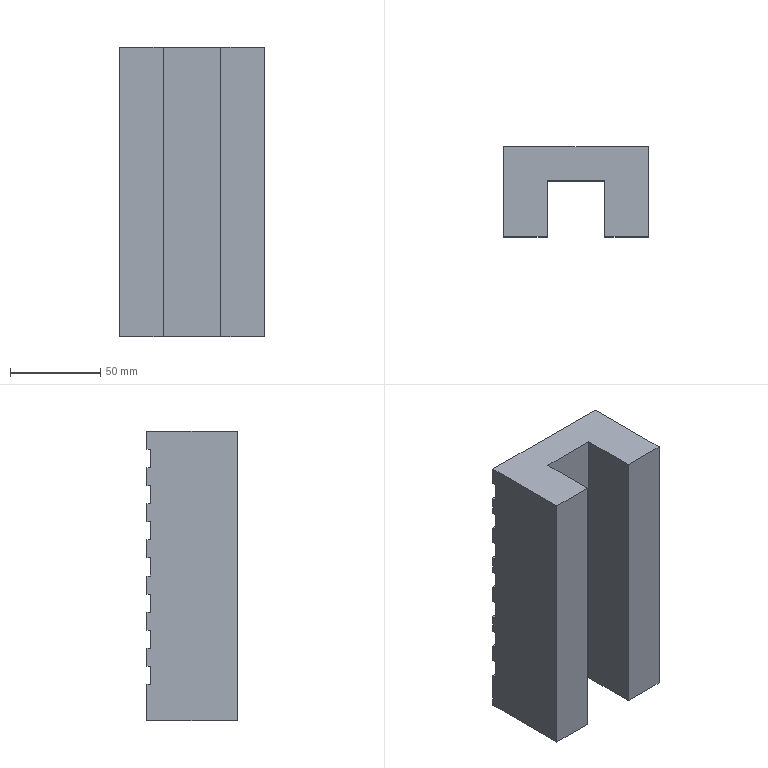Part | SolidWorks | features Extrusion 1, ICE 1, LPattern 1 | 1 solid | 38 faces | box 80 x 50 x 160 mm | volume 470080 mm3 | plane 38
STEP:
#1=CARTESIAN_POINT('',(40.,25.,40.));
#2=VERTEX_POINT('',#1);
#3=CARTESIAN_POINT('',(-40.,25.,40.));
#4=VERTEX_POINT('',#3);
#5=CARTESIAN_POINT('',(-40.,25.,40.));
#6=DIRECTION('',(-1.,0.,0.));
#7=VECTOR('',#6,1000.);
#8=LINE('',#5,#7);
#9=EDGE_CURVE('',#2,#4,#8,.T.);
#10=ORIENTED_EDGE('',*,*,#9,.F.);
#11=CARTESIAN_POINT('',(40.,25.,30.));
#12=VERTEX_POINT('',#11);
#13=CARTESIAN_POINT('',(40.,25.,160.));
#14=DIRECTION('',(0.,0.,-1.));
#15=VECTOR('',#14,1000.);
#16=LINE('',#13,#15);
#17=EDGE_CURVE('',#2,#12,#16,.T.);
#18=ORIENTED_EDGE('',*,*,#17,.T.);
#19=CARTESIAN_POINT('',(-40.,25.,30.));
#20=VERTEX_POINT('',#19);
#21=CARTESIAN_POINT('',(-40.,25.,30.));
#22=DIRECTION('',(1.,0.,0.));
#23=VECTOR('',#22,1000.);
#24=LINE('',#21,#23);
#25=EDGE_CURVE('',#20,#12,#24,.T.);
#26=ORIENTED_EDGE('',*,*,#25,.F.);
#27=CARTESIAN_POINT('',(-40.,25.,160.));
#28=DIRECTION('',(0.,0.,-1.));
#29=VECTOR('',#28,1000.);
#30=LINE('',#27,#29);
#31=EDGE_CURVE('',#4,#20,#30,.T.);
#32=ORIENTED_EDGE('',*,*,#31,.F.);
#33=EDGE_LOOP('',(#10,#18,#26,#32));
#34=FACE_OUTER_BOUND('',#33,.T.);
#35=CARTESIAN_POINT('',(0.,25.,160.));
#36=DIRECTION('',(0.,1.,0.));
#37=DIRECTION('',(-1.,0.,0.));
#38=AXIS2_PLACEMENT_3D('',#35,#36,#37);
#39=PLANE('',#38);
#40=ADVANCED_FACE('',(#34),#39,.T.);
#41=CARTESIAN_POINT('',(-40.,25.,50.));
#42=VERTEX_POINT('',#41);
#43=CARTESIAN_POINT('',(40.,25.,50.));
#44=VERTEX_POINT('',#43);
#45=CARTESIAN_POINT('',(-40.,25.,50.));
#46=DIRECTION('',(1.,0.,0.));
#47=VECTOR('',#46,1000.);
#48=LINE('',#45,#47);
#49=EDGE_CURVE('',#42,#44,#48,.T.);
#50=ORIENTED_EDGE('',*,*,#49,.F.);
#51=CARTESIAN_POINT('',(-40.,25.,60.));
#52=VERTEX_POINT('',#51);
#53=CARTESIAN_POINT('',(-40.,25.,160.));
#54=DIRECTION('',(0.,0.,-1.));
#55=VECTOR('',#54,1000.);
#56=LINE('',#53,#55);
#57=EDGE_CURVE('',#52,#42,#56,.T.);
#58=ORIENTED_EDGE('',*,*,#57,.F.);
#59=CARTESIAN_POINT('',(40.,25.,60.));
#60=VERTEX_POINT('',#59);
#61=CARTESIAN_POINT('',(-40.,25.,60.));
#62=DIRECTION('',(-1.,0.,0.));
#63=VECTOR('',#62,1000.);
#64=LINE('',#61,#63);
#65=EDGE_CURVE('',#60,#52,#64,.T.);
#66=ORIENTED_EDGE('',*,*,#65,.F.);
#67=CARTESIAN_POINT('',(40.,25.,160.));
#68=DIRECTION('',(0.,0.,-1.));
#69=VECTOR('',#68,1000.);
#70=LINE('',#67,#69);
#71=EDGE_CURVE('',#60,#44,#70,.T.);
#72=ORIENTED_EDGE('',*,*,#71,.T.);
#73=EDGE_LOOP('',(#50,#58,#66,#72));
#74=FACE_OUTER_BOUND('',#73,.T.);
#75=CARTESIAN_POINT('',(0.,25.,160.));
#76=DIRECTION('',(0.,1.,0.));
#77=DIRECTION('',(-1.,0.,0.));
#78=AXIS2_PLACEMENT_3D('',#75,#76,#77);
#79=PLANE('',#78);
#80=ADVANCED_FACE('',(#74),#79,.T.);
#81=CARTESIAN_POINT('',(-40.,25.,70.));
#82=VERTEX_POINT('',#81);
#83=CARTESIAN_POINT('',(40.,25.,70.));
#84=VERTEX_POINT('',#83);
#85=CARTESIAN_POINT('',(-40.,25.,70.));
#86=DIRECTION('',(1.,0.,0.));
#87=VECTOR('',#86,1000.);
#88=LINE('',#85,#87);
#89=EDGE_CURVE('',#82,#84,#88,.T.);
#90=ORIENTED_EDGE('',*,*,#89,.F.);
#91=CARTESIAN_POINT('',(-40.,25.,80.));
#92=VERTEX_POINT('',#91);
#93=CARTESIAN_POINT('',(-40.,25.,160.));
#94=DIRECTION('',(0.,0.,-1.));
#95=VECTOR('',#94,1000.);
#96=LINE('',#93,#95);
#97=EDGE_CURVE('',#92,#82,#96,.T.);
#98=ORIENTED_EDGE('',*,*,#97,.F.);
#99=CARTESIAN_POINT('',(40.,25.,80.));
#100=VERTEX_POINT('',#99);
#101=CARTESIAN_POINT('',(-40.,25.,80.));
#102=DIRECTION('',(-1.,0.,0.));
#103=VECTOR('',#102,1000.);
#104=LINE('',#101,#103);
#105=EDGE_CURVE('',#100,#92,#104,.T.);
#106=ORIENTED_EDGE('',*,*,#105,.F.);
#107=CARTESIAN_POINT('',(40.,25.,160.));
#108=DIRECTION('',(0.,0.,-1.));
#109=VECTOR('',#108,1000.);
#110=LINE('',#107,#109);
#111=EDGE_CURVE('',#100,#84,#110,.T.);
#112=ORIENTED_EDGE('',*,*,#111,.T.);
#113=EDGE_LOOP('',(#90,#98,#106,#112));
#114=FACE_OUTER_BOUND('',#113,.T.);
#115=CARTESIAN_POINT('',(0.,25.,160.));
#116=DIRECTION('',(0.,1.,0.));
#117=DIRECTION('',(-1.,0.,0.));
#118=AXIS2_PLACEMENT_3D('',#115,#116,#117);
#119=PLANE('',#118);
#120=ADVANCED_FACE('',(#114),#119,.T.);
#121=CARTESIAN_POINT('',(-40.,25.,90.));
#122=VERTEX_POINT('',#121);
#123=CARTESIAN_POINT('',(40.,25.,90.));
#124=VERTEX_POINT('',#123);
#125=CARTESIAN_POINT('',(-40.,25.,90.));
#126=DIRECTION('',(1.,0.,0.));
#127=VECTOR('',#126,1000.);
#128=LINE('',#125,#127);
#129=EDGE_CURVE('',#122,#124,#128,.T.);
#130=ORIENTED_EDGE('',*,*,#129,.F.);
#131=CARTESIAN_POINT('',(-40.,25.,100.));
#132=VERTEX_POINT('',#131);
#133=CARTESIAN_POINT('',(-40.,25.,160.));
#134=DIRECTION('',(0.,0.,-1.));
#135=VECTOR('',#134,1000.);
#136=LINE('',#133,#135);
#137=EDGE_CURVE('',#132,#122,#136,.T.);
#138=ORIENTED_EDGE('',*,*,#137,.F.);
#139=CARTESIAN_POINT('',(40.,25.,100.));
#140=VERTEX_POINT('',#139);
#141=CARTESIAN_POINT('',(-40.,25.,100.));
#142=DIRECTION('',(-1.,0.,0.));
#143=VECTOR('',#142,1000.);
#144=LINE('',#141,#143);
#145=EDGE_CURVE('',#140,#132,#144,.T.);
#146=ORIENTED_EDGE('',*,*,#145,.F.);
#147=CARTESIAN_POINT('',(40.,25.,160.));
#148=DIRECTION('',(0.,0.,-1.));
#149=VECTOR('',#148,1000.);
#150=LINE('',#147,#149);
#151=EDGE_CURVE('',#140,#124,#150,.T.);
#152=ORIENTED_EDGE('',*,*,#151,.T.);
#153=EDGE_LOOP('',(#130,#138,#146,#152));
#154=FACE_OUTER_BOUND('',#153,.T.);
#155=CARTESIAN_POINT('',(0.,25.,160.));
#156=DIRECTION('',(0.,1.,0.));
#157=DIRECTION('',(-1.,0.,0.));
#158=AXIS2_PLACEMENT_3D('',#155,#156,#157);
#159=PLANE('',#158);
#160=ADVANCED_FACE('',(#154),#159,.T.);
#161=CARTESIAN_POINT('',(-40.,25.,110.));
#162=VERTEX_POINT('',#161);
#163=CARTESIAN_POINT('',(40.,25.,110.));
#164=VERTEX_POINT('',#163);
#165=CARTESIAN_POINT('',(-40.,25.,110.));
#166=DIRECTION('',(1.,0.,0.));
#167=VECTOR('',#166,1000.);
#168=LINE('',#165,#167);
#169=EDGE_CURVE('',#162,#164,#168,.T.);
#170=ORIENTED_EDGE('',*,*,#169,.F.);
#171=CARTESIAN_POINT('',(-40.,25.,120.));
#172=VERTEX_POINT('',#171);
#173=CARTESIAN_POINT('',(-40.,25.,160.));
#174=DIRECTION('',(0.,0.,-1.));
#175=VECTOR('',#174,1000.);
#176=LINE('',#173,#175);
#177=EDGE_CURVE('',#172,#162,#176,.T.);
#178=ORIENTED_EDGE('',*,*,#177,.F.);
#179=CARTESIAN_POINT('',(40.,25.,120.));
#180=VERTEX_POINT('',#179);
#181=CARTESIAN_POINT('',(-40.,25.,120.));
#182=DIRECTION('',(-1.,0.,0.));
#183=VECTOR('',#182,1000.);
#184=LINE('',#181,#183);
#185=EDGE_CURVE('',#180,#172,#184,.T.);
#186=ORIENTED_EDGE('',*,*,#185,.F.);
#187=CARTESIAN_POINT('',(40.,25.,160.));
#188=DIRECTION('',(0.,0.,-1.));
#189=VECTOR('',#188,1000.);
#190=LINE('',#187,#189);
#191=EDGE_CURVE('',#180,#164,#190,.T.);
#192=ORIENTED_EDGE('',*,*,#191,.T.);
#193=EDGE_LOOP('',(#170,#178,#186,#192));
#194=FACE_OUTER_BOUND('',#193,.T.);
#195=CARTESIAN_POINT('',(0.,25.,160.));
#196=DIRECTION('',(0.,1.,0.));
#197=DIRECTION('',(-1.,0.,0.));
#198=AXIS2_PLACEMENT_3D('',#195,#196,#197);
#199=PLANE('',#198);
#200=ADVANCED_FACE('',(#194),#199,.T.);
#201=CARTESIAN_POINT('',(-40.,25.,130.));
#202=VERTEX_POINT('',#201);
#203=CARTESIAN_POINT('',(40.,25.,130.));
#204=VERTEX_POINT('',#203);
#205=CARTESIAN_POINT('',(-40.,25.,130.));
#206=DIRECTION('',(1.,0.,0.));
#207=VECTOR('',#206,1000.);
#208=LINE('',#205,#207);
#209=EDGE_CURVE('',#202,#204,#208,.T.);
#210=ORIENTED_EDGE('',*,*,#209,.F.);
#211=CARTESIAN_POINT('',(-40.,25.,140.));
#212=VERTEX_POINT('',#211);
#213=CARTESIAN_POINT('',(-40.,25.,160.));
#214=DIRECTION('',(0.,0.,-1.));
#215=VECTOR('',#214,1000.);
#216=LINE('',#213,#215);
#217=EDGE_CURVE('',#212,#202,#216,.T.);
#218=ORIENTED_EDGE('',*,*,#217,.F.);
#219=CARTESIAN_POINT('',(40.,25.,140.));
#220=VERTEX_POINT('',#219);
#221=CARTESIAN_POINT('',(-40.,25.,140.));
#222=DIRECTION('',(-1.,0.,0.));
#223=VECTOR('',#222,1000.);
#224=LINE('',#221,#223);
#225=EDGE_CURVE('',#220,#212,#224,.T.);
#226=ORIENTED_EDGE('',*,*,#225,.F.);
#227=CARTESIAN_POINT('',(40.,25.,160.));
#228=DIRECTION('',(0.,0.,-1.));
#229=VECTOR('',#228,1000.);
#230=LINE('',#227,#229);
#231=EDGE_CURVE('',#220,#204,#230,.T.);
#232=ORIENTED_EDGE('',*,*,#231,.T.);
#233=EDGE_LOOP('',(#210,#218,#226,#232));
#234=FACE_OUTER_BOUND('',#233,.T.);
#235=CARTESIAN_POINT('',(0.,25.,160.));
#236=DIRECTION('',(0.,1.,0.));
#237=DIRECTION('',(-1.,0.,0.));
#238=AXIS2_PLACEMENT_3D('',#235,#236,#237);
#239=PLANE('',#238);
#240=ADVANCED_FACE('',(#234),#239,.T.);
#241=CARTESIAN_POINT('',(40.,25.,20.));
#242=VERTEX_POINT('',#241);
#243=CARTESIAN_POINT('',(-40.,25.,20.));
#244=VERTEX_POINT('',#243);
#245=CARTESIAN_POINT('',(-40.,25.,20.));
#246=DIRECTION('',(-1.,0.,0.));
#247=VECTOR('',#246,1000.);
#248=LINE('',#245,#247);
#249=EDGE_CURVE('',#242,#244,#248,.T.);
#250=ORIENTED_EDGE('',*,*,#249,.F.);
#251=CARTESIAN_POINT('',(40.,25.,0.));
#252=VERTEX_POINT('',#251);
#253=CARTESIAN_POINT('',(40.,25.,160.));
#254=DIRECTION('',(0.,0.,-1.));
#255=VECTOR('',#254,1000.);
#256=LINE('',#253,#255);
#257=EDGE_CURVE('',#242,#252,#256,.T.);
#258=ORIENTED_EDGE('',*,*,#257,.T.);
#259=CARTESIAN_POINT('',(-40.,25.,0.));
#260=VERTEX_POINT('',#259);
#261=CARTESIAN_POINT('',(0.,25.,0.));
#262=DIRECTION('',(1.,0.,0.));
#263=VECTOR('',#262,1000.);
#264=LINE('',#261,#263);
#265=EDGE_CURVE('',#260,#252,#264,.T.);
#266=ORIENTED_EDGE('',*,*,#265,.F.);
#267=CARTESIAN_POINT('',(-40.,25.,160.));
#268=DIRECTION('',(0.,0.,-1.));
#269=VECTOR('',#268,1000.);
#270=LINE('',#267,#269);
#271=EDGE_CURVE('',#244,#260,#270,.T.);
#272=ORIENTED_EDGE('',*,*,#271,.F.);
#273=EDGE_LOOP('',(#250,#258,#266,#272));
#274=FACE_OUTER_BOUND('',#273,.T.);
#275=CARTESIAN_POINT('',(0.,25.,160.));
#276=DIRECTION('',(0.,1.,0.));
#277=DIRECTION('',(-1.,0.,0.));
#278=AXIS2_PLACEMENT_3D('',#275,#276,#277);
#279=PLANE('',#278);
#280=ADVANCED_FACE('',(#274),#279,.T.);
#281=CARTESIAN_POINT('',(-16.,-25.,0.));
#282=VERTEX_POINT('',#281);
#283=CARTESIAN_POINT('',(-16.,6.,0.));
#284=VERTEX_POINT('',#283);
#285=CARTESIAN_POINT('',(-16.,0.,0.));
#286=DIRECTION('',(0.,1.,0.));
#287=VECTOR('',#286,1000.);
#288=LINE('',#285,#287);
#289=EDGE_CURVE('',#282,#284,#288,.T.);
#290=ORIENTED_EDGE('',*,*,#289,.T.);
#291=CARTESIAN_POINT('',(-16.,6.,160.));
#292=VERTEX_POINT('',#291);
#293=CARTESIAN_POINT('',(-16.,6.,160.));
#294=DIRECTION('',(0.,0.,-1.));
#295=VECTOR('',#294,1000.);
#296=LINE('',#293,#295);
#297=EDGE_CURVE('',#292,#284,#296,.T.);
#298=ORIENTED_EDGE('',*,*,#297,.F.);
#299=CARTESIAN_POINT('',(-16.,-25.,160.));
#300=VERTEX_POINT('',#299);
#301=CARTESIAN_POINT('',(-16.,0.,160.));
#302=DIRECTION('',(0.,1.,0.));
#303=VECTOR('',#302,1000.);
#304=LINE('',#301,#303);
#305=EDGE_CURVE('',#300,#292,#304,.T.);
#306=ORIENTED_EDGE('',*,*,#305,.F.);
#307=CARTESIAN_POINT('',(-16.,-25.,160.));
#308=DIRECTION('',(0.,0.,-1.));
#309=VECTOR('',#308,1000.);
#310=LINE('',#307,#309);
#311=EDGE_CURVE('',#300,#282,#310,.T.);
#312=ORIENTED_EDGE('',*,*,#311,.T.);
#313=EDGE_LOOP('',(#290,#298,#306,#312));
#314=FACE_OUTER_BOUND('',#313,.T.);
#315=CARTESIAN_POINT('',(-16.,0.,160.));
#316=DIRECTION('',(-1.,0.,0.));
#317=DIRECTION('',(0.,0.,1.));
#318=AXIS2_PLACEMENT_3D('',#315,#316,#317);
#319=PLANE('',#318);
#320=ADVANCED_FACE('',(#314),#319,.F.);
#321=CARTESIAN_POINT('',(16.,6.,0.));
#322=VERTEX_POINT('',#321);
#323=CARTESIAN_POINT('',(0.,6.,0.));
#324=DIRECTION('',(1.,0.,0.));
#325=VECTOR('',#324,1000.);
#326=LINE('',#323,#325);
#327=EDGE_CURVE('',#284,#322,#326,.T.);
#328=ORIENTED_EDGE('',*,*,#327,.T.);
#329=CARTESIAN_POINT('',(16.,6.,160.));
#330=VERTEX_POINT('',#329);
#331=CARTESIAN_POINT('',(16.,6.,160.));
#332=DIRECTION('',(0.,0.,-1.));
#333=VECTOR('',#332,1000.);
#334=LINE('',#331,#333);
#335=EDGE_CURVE('',#330,#322,#334,.T.);
#336=ORIENTED_EDGE('',*,*,#335,.F.);
#337=CARTESIAN_POINT('',(0.,6.,160.));
#338=DIRECTION('',(1.,0.,0.));
#339=VECTOR('',#338,1000.);
#340=LINE('',#337,#339);
#341=EDGE_CURVE('',#292,#330,#340,.T.);
#342=ORIENTED_EDGE('',*,*,#341,.F.);
#343=ORIENTED_EDGE('',*,*,#297,.T.);
#344=EDGE_LOOP('',(#328,#336,#342,#343));
#345=FACE_OUTER_BOUND('',#344,.T.);
#346=CARTESIAN_POINT('',(0.,6.,160.));
#347=DIRECTION('',(0.,1.,0.));
#348=DIRECTION('',(-1.,0.,0.));
#349=AXIS2_PLACEMENT_3D('',#346,#347,#348);
#350=PLANE('',#349);
#351=ADVANCED_FACE('',(#345),#350,.F.);
#352=CARTESIAN_POINT('',(16.,-25.,0.));
#353=VERTEX_POINT('',#352);
#354=CARTESIAN_POINT('',(16.,0.,0.));
#355=DIRECTION('',(0.,1.,0.));
#356=VECTOR('',#355,1000.);
#357=LINE('',#354,#356);
#358=EDGE_CURVE('',#353,#322,#357,.T.);
#359=ORIENTED_EDGE('',*,*,#358,.F.);
#360=CARTESIAN_POINT('',(16.,-25.,160.));
#361=VERTEX_POINT('',#360);
#362=CARTESIAN_POINT('',(16.,-25.,160.));
#363=DIRECTION('',(0.,0.,-1.));
#364=VECTOR('',#363,1000.);
#365=LINE('',#362,#364);
#366=EDGE_CURVE('',#361,#353,#365,.T.);
#367=ORIENTED_EDGE('',*,*,#366,.F.);
#368=CARTESIAN_POINT('',(16.,0.,160.));
#369=DIRECTION('',(0.,1.,0.));
#370=VECTOR('',#369,1000.);
#371=LINE('',#368,#370);
#372=EDGE_CURVE('',#361,#330,#371,.T.);
#373=ORIENTED_EDGE('',*,*,#372,.T.);
#374=ORIENTED_EDGE('',*,*,#335,.T.);
#375=EDGE_LOOP('',(#359,#367,#373,#374));
#376=FACE_OUTER_BOUND('',#375,.T.);
#377=CARTESIAN_POINT('',(16.,0.,160.));
#378=DIRECTION('',(-1.,0.,0.));
#379=DIRECTION('',(0.,-1.,0.));
#380=AXIS2_PLACEMENT_3D('',#377,#378,#379);
#381=PLANE('',#380);
#382=ADVANCED_FACE('',(#376),#381,.T.);
#383=CARTESIAN_POINT('',(40.,-25.,0.));
#384=VERTEX_POINT('',#383);
#385=CARTESIAN_POINT('',(0.,-25.,0.));
#386=DIRECTION('',(1.,0.,0.));
#387=VECTOR('',#386,1000.);
#388=LINE('',#385,#387);
#389=EDGE_CURVE('',#353,#384,#388,.T.);
#390=ORIENTED_EDGE('',*,*,#389,.T.);
#391=CARTESIAN_POINT('',(40.,-25.,160.));
#392=VERTEX_POINT('',#391);
#393=CARTESIAN_POINT('',(40.,-25.,160.));
#394=DIRECTION('',(0.,0.,-1.));
#395=VECTOR('',#394,1000.);
#396=LINE('',#393,#395);
#397=EDGE_CURVE('',#392,#384,#396,.T.);
#398=ORIENTED_EDGE('',*,*,#397,.F.);
#399=CARTESIAN_POINT('',(0.,-25.,160.));
#400=DIRECTION('',(1.,0.,0.));
#401=VECTOR('',#400,1000.);
#402=LINE('',#399,#401);
#403=EDGE_CURVE('',#361,#392,#402,.T.);
#404=ORIENTED_EDGE('',*,*,#403,.F.);
#405=ORIENTED_EDGE('',*,*,#366,.T.);
#406=EDGE_LOOP('',(#390,#398,#404,#405));
#407=FACE_OUTER_BOUND('',#406,.T.);
#408=CARTESIAN_POINT('',(0.,-25.,160.));
#409=DIRECTION('',(0.,1.,0.));
#410=DIRECTION('',(-1.,0.,0.));
#411=AXIS2_PLACEMENT_3D('',#408,#409,#410);
#412=PLANE('',#411);
#413=ADVANCED_FACE('',(#407),#412,.F.);
#414=CARTESIAN_POINT('',(40.,23.,40.));
#415=VERTEX_POINT('',#414);
#416=CARTESIAN_POINT('',(40.,23.,40.));
#417=DIRECTION('',(0.,1.,0.));
#418=VECTOR('',#417,1000.);
#419=LINE('',#416,#418);
#420=EDGE_CURVE('',#415,#2,#419,.T.);
#421=ORIENTED_EDGE('',*,*,#420,.F.);
#422=CARTESIAN_POINT('',(40.,23.,50.));
#423=VERTEX_POINT('',#422);
#424=CARTESIAN_POINT('',(40.,23.,40.));
#425=DIRECTION('',(0.,0.,-1.));
#426=VECTOR('',#425,1000.);
#427=LINE('',#424,#426);
#428=EDGE_CURVE('',#423,#415,#427,.T.);
#429=ORIENTED_EDGE('',*,*,#428,.F.);
#430=CARTESIAN_POINT('',(40.,23.,50.));
#431=DIRECTION('',(0.,1.,0.));
#432=VECTOR('',#431,1000.);
#433=LINE('',#430,#432);
#434=EDGE_CURVE('',#423,#44,#433,.T.);
#435=ORIENTED_EDGE('',*,*,#434,.T.);
#436=ORIENTED_EDGE('',*,*,#71,.F.);
#437=CARTESIAN_POINT('',(40.,23.,60.));
#438=VERTEX_POINT('',#437);
#439=CARTESIAN_POINT('',(40.,23.,60.));
#440=DIRECTION('',(0.,1.,0.));
#441=VECTOR('',#440,1000.);
#442=LINE('',#439,#441);
#443=EDGE_CURVE('',#438,#60,#442,.T.);
#444=ORIENTED_EDGE('',*,*,#443,.F.);
#445=CARTESIAN_POINT('',(40.,23.,70.));
#446=VERTEX_POINT('',#445);
#447=CARTESIAN_POINT('',(40.,23.,60.));
#448=DIRECTION('',(0.,0.,-1.));
#449=VECTOR('',#448,1000.);
#450=LINE('',#447,#449);
#451=EDGE_CURVE('',#446,#438,#450,.T.);
#452=ORIENTED_EDGE('',*,*,#451,.F.);
#453=CARTESIAN_POINT('',(40.,23.,70.));
#454=DIRECTION('',(0.,1.,0.));
#455=VECTOR('',#454,1000.);
#456=LINE('',#453,#455);
#457=EDGE_CURVE('',#446,#84,#456,.T.);
#458=ORIENTED_EDGE('',*,*,#457,.T.);
#459=ORIENTED_EDGE('',*,*,#111,.F.);
#460=CARTESIAN_POINT('',(40.,23.,80.));
#461=VERTEX_POINT('',#460);
#462=CARTESIAN_POINT('',(40.,23.,80.));
#463=DIRECTION('',(0.,1.,0.));
#464=VECTOR('',#463,1000.);
#465=LINE('',#462,#464);
#466=EDGE_CURVE('',#461,#100,#465,.T.);
#467=ORIENTED_EDGE('',*,*,#466,.F.);
#468=CARTESIAN_POINT('',(40.,23.,90.));
#469=VERTEX_POINT('',#468);
#470=CARTESIAN_POINT('',(40.,23.,80.));
#471=DIRECTION('',(0.,0.,-1.));
#472=VECTOR('',#471,1000.);
#473=LINE('',#470,#472);
#474=EDGE_CURVE('',#469,#461,#473,.T.);
#475=ORIENTED_EDGE('',*,*,#474,.F.);
#476=CARTESIAN_POINT('',(40.,23.,90.));
#477=DIRECTION('',(0.,1.,0.));
#478=VECTOR('',#477,1000.);
#479=LINE('',#476,#478);
#480=EDGE_CURVE('',#469,#124,#479,.T.);
#481=ORIENTED_EDGE('',*,*,#480,.T.);
#482=ORIENTED_EDGE('',*,*,#151,.F.);
#483=CARTESIAN_POINT('',(40.,23.,100.));
#484=VERTEX_POINT('',#483);
#485=CARTESIAN_POINT('',(40.,23.,100.));
#486=DIRECTION('',(0.,1.,0.));
#487=VECTOR('',#486,1000.);
#488=LINE('',#485,#487);
#489=EDGE_CURVE('',#484,#140,#488,.T.);
#490=ORIENTED_EDGE('',*,*,#489,.F.);
#491=CARTESIAN_POINT('',(40.,23.,110.));
#492=VERTEX_POINT('',#491);
#493=CARTESIAN_POINT('',(40.,23.,100.));
#494=DIRECTION('',(0.,0.,-1.));
#495=VECTOR('',#494,1000.);
#496=LINE('',#493,#495);
#497=EDGE_CURVE('',#492,#484,#496,.T.);
#498=ORIENTED_EDGE('',*,*,#497,.F.);
#499=CARTESIAN_POINT('',(40.,23.,110.));
#500=DIRECTION('',(0.,1.,0.));
#501=VECTOR('',#500,1000.);
#502=LINE('',#499,#501);
#503=EDGE_CURVE('',#492,#164,#502,.T.);
#504=ORIENTED_EDGE('',*,*,#503,.T.);
#505=ORIENTED_EDGE('',*,*,#191,.F.);
#506=CARTESIAN_POINT('',(40.,23.,120.));
#507=VERTEX_POINT('',#506);
#508=CARTESIAN_POINT('',(40.,23.,120.));
#509=DIRECTION('',(0.,1.,0.));
#510=VECTOR('',#509,1000.);
#511=LINE('',#508,#510);
#512=EDGE_CURVE('',#507,#180,#511,.T.);
#513=ORIENTED_EDGE('',*,*,#512,.F.);
#514=CARTESIAN_POINT('',(40.,23.,130.));
#515=VERTEX_POINT('',#514);
#516=CARTESIAN_POINT('',(40.,23.,120.));
#517=DIRECTION('',(0.,0.,-1.));
#518=VECTOR('',#517,1000.);
#519=LINE('',#516,#518);
#520=EDGE_CURVE('',#515,#507,#519,.T.);
#521=ORIENTED_EDGE('',*,*,#520,.F.);
#522=CARTESIAN_POINT('',(40.,23.,130.));
#523=DIRECTION('',(0.,1.,0.));
#524=VECTOR('',#523,1000.);
#525=LINE('',#522,#524);
#526=EDGE_CURVE('',#515,#204,#525,.T.);
#527=ORIENTED_EDGE('',*,*,#526,.T.);
#528=ORIENTED_EDGE('',*,*,#231,.F.);
#529=CARTESIAN_POINT('',(40.,23.,140.));
#530=VERTEX_POINT('',#529);
#531=CARTESIAN_POINT('',(40.,23.,140.));
#532=DIRECTION('',(0.,1.,0.));
#533=VECTOR('',#532,1000.);
#534=LINE('',#531,#533);
#535=EDGE_CURVE('',#530,#220,#534,.T.);
#536=ORIENTED_EDGE('',*,*,#535,.F.);
#537=CARTESIAN_POINT('',(40.,23.,150.));
#538=VERTEX_POINT('',#537);
#539=CARTESIAN_POINT('',(40.,23.,140.));
#540=DIRECTION('',(0.,0.,-1.));
#541=VECTOR('',#540,1000.);
#542=LINE('',#539,#541);
#543=EDGE_CURVE('',#538,#530,#542,.T.);
#544=ORIENTED_EDGE('',*,*,#543,.F.);
#545=CARTESIAN_POINT('',(40.,25.,150.));
#546=VERTEX_POINT('',#545);
#547=CARTESIAN_POINT('',(40.,23.,150.));
#548=DIRECTION('',(0.,1.,0.));
#549=VECTOR('',#548,1000.);
#550=LINE('',#547,#549);
#551=EDGE_CURVE('',#538,#546,#550,.T.);
#552=ORIENTED_EDGE('',*,*,#551,.T.);
#553=CARTESIAN_POINT('',(40.,25.,160.));
#554=VERTEX_POINT('',#553);
#555=CARTESIAN_POINT('',(40.,25.,160.));
#556=DIRECTION('',(0.,0.,-1.));
#557=VECTOR('',#556,1000.);
#558=LINE('',#555,#557);
#559=EDGE_CURVE('',#554,#546,#558,.T.);
#560=ORIENTED_EDGE('',*,*,#559,.F.);
#561=CARTESIAN_POINT('',(40.,0.,160.));
#562=DIRECTION('',(0.,-1.,0.));
#563=VECTOR('',#562,1000.);
#564=LINE('',#561,#563);
#565=EDGE_CURVE('',#554,#392,#564,.T.);
#566=ORIENTED_EDGE('',*,*,#565,.T.);
#567=ORIENTED_EDGE('',*,*,#397,.T.);
#568=CARTESIAN_POINT('',(40.,0.,0.));
#569=DIRECTION('',(0.,-1.,0.));
#570=VECTOR('',#569,1000.);
#571=LINE('',#568,#570);
#572=EDGE_CURVE('',#252,#384,#571,.T.);
#573=ORIENTED_EDGE('',*,*,#572,.F.);
#574=ORIENTED_EDGE('',*,*,#257,.F.);
#575=CARTESIAN_POINT('',(40.,23.,20.));
#576=VERTEX_POINT('',#575);
#577=CARTESIAN_POINT('',(40.,23.,20.));
#578=DIRECTION('',(0.,1.,0.));
#579=VECTOR('',#578,1000.);
#580=LINE('',#577,#579);
#581=EDGE_CURVE('',#576,#242,#580,.T.);
#582=ORIENTED_EDGE('',*,*,#581,.F.);
#583=CARTESIAN_POINT('',(40.,23.,30.));
#584=VERTEX_POINT('',#583);
#585=CARTESIAN_POINT('',(40.,23.,20.));
#586=DIRECTION('',(0.,0.,-1.));
#587=VECTOR('',#586,1000.);
#588=LINE('',#585,#587);
#589=EDGE_CURVE('',#584,#576,#588,.T.);
#590=ORIENTED_EDGE('',*,*,#589,.F.);
#591=CARTESIAN_POINT('',(40.,23.,30.));
#592=DIRECTION('',(0.,1.,0.));
#593=VECTOR('',#592,1000.);
#594=LINE('',#591,#593);
#595=EDGE_CURVE('',#584,#12,#594,.T.);
#596=ORIENTED_EDGE('',*,*,#595,.T.);
#597=ORIENTED_EDGE('',*,*,#17,.F.);
#598=EDGE_LOOP('',(#421,#429,#435,#436,#444,#452,#458,#459,#467,#475,#481,#482,#490,#498,#504,#505,#513,#521,#527,#528,#536,#544,#552,#560,#566,#567,#573,#574,#582,#590,#596,#597));
#599=FACE_OUTER_BOUND('',#598,.T.);
#600=CARTESIAN_POINT('',(40.,0.,160.));
#601=DIRECTION('',(1.,0.,0.));
#602=DIRECTION('',(0.,1.,0.));
#603=AXIS2_PLACEMENT_3D('',#600,#601,#602);
#604=PLANE('',#603);
#605=ADVANCED_FACE('',(#599),#604,.T.);
#606=CARTESIAN_POINT('',(-40.,25.,150.));
#607=VERTEX_POINT('',#606);
#608=CARTESIAN_POINT('',(-40.,25.,150.));
#609=DIRECTION('',(1.,0.,0.));
#610=VECTOR('',#609,1000.);
#611=LINE('',#608,#610);
#612=EDGE_CURVE('',#607,#546,#611,.T.);
#613=ORIENTED_EDGE('',*,*,#612,.F.);
#614=CARTESIAN_POINT('',(-40.,25.,160.));
#615=VERTEX_POINT('',#614);
#616=CARTESIAN_POINT('',(-40.,25.,160.));
#617=DIRECTION('',(0.,0.,-1.));
#618=VECTOR('',#617,1000.);
#619=LINE('',#616,#618);
#620=EDGE_CURVE('',#615,#607,#619,.T.);
#621=ORIENTED_EDGE('',*,*,#620,.F.);
#622=CARTESIAN_POINT('',(0.,25.,160.));
#623=DIRECTION('',(1.,0.,0.));
#624=VECTOR('',#623,1000.);
#625=LINE('',#622,#624);
#626=EDGE_CURVE('',#615,#554,#625,.T.);
#627=ORIENTED_EDGE('',*,*,#626,.T.);
#628=ORIENTED_EDGE('',*,*,#559,.T.);
#629=EDGE_LOOP('',(#613,#621,#627,#628));
#630=FACE_OUTER_BOUND('',#629,.T.);
#631=CARTESIAN_POINT('',(0.,25.,160.));
#632=DIRECTION('',(0.,1.,0.));
#633=DIRECTION('',(-1.,0.,0.));
#634=AXIS2_PLACEMENT_3D('',#631,#632,#633);
#635=PLANE('',#634);
#636=ADVANCED_FACE('',(#630),#635,.T.);
#637=CARTESIAN_POINT('',(-40.,23.,40.));
#638=VERTEX_POINT('',#637);
#639=CARTESIAN_POINT('',(-40.,23.,50.));
#640=VERTEX_POINT('',#639);
#641=CARTESIAN_POINT('',(-40.,23.,40.));
#642=DIRECTION('',(0.,0.,1.));
#643=VECTOR('',#642,1000.);
#644=LINE('',#641,#643);
#645=EDGE_CURVE('',#638,#640,#644,.T.);
#646=ORIENTED_EDGE('',*,*,#645,.F.);
#647=CARTESIAN_POINT('',(-40.,23.,40.));
#648=DIRECTION('',(0.,1.,0.));
#649=VECTOR('',#648,1000.);
#650=LINE('',#647,#649);
#651=EDGE_CURVE('',#638,#4,#650,.T.);
#652=ORIENTED_EDGE('',*,*,#651,.T.);
#653=ORIENTED_EDGE('',*,*,#31,.T.);
#654=CARTESIAN_POINT('',(-40.,23.,30.));
#655=VERTEX_POINT('',#654);
#656=CARTESIAN_POINT('',(-40.,23.,30.));
#657=DIRECTION('',(0.,1.,0.));
#658=VECTOR('',#657,1000.);
#659=LINE('',#656,#658);
#660=EDGE_CURVE('',#655,#20,#659,.T.);
#661=ORIENTED_EDGE('',*,*,#660,.F.);
#662=CARTESIAN_POINT('',(-40.,23.,20.));
#663=VERTEX_POINT('',#662);
#664=CARTESIAN_POINT('',(-40.,23.,20.));
#665=DIRECTION('',(0.,0.,1.));
#666=VECTOR('',#665,1000.);
#667=LINE('',#664,#666);
#668=EDGE_CURVE('',#663,#655,#667,.T.);
#669=ORIENTED_EDGE('',*,*,#668,.F.);
#670=CARTESIAN_POINT('',(-40.,23.,20.));
#671=DIRECTION('',(0.,1.,0.));
#672=VECTOR('',#671,1000.);
#673=LINE('',#670,#672);
#674=EDGE_CURVE('',#663,#244,#673,.T.);
#675=ORIENTED_EDGE('',*,*,#674,.T.);
#676=ORIENTED_EDGE('',*,*,#271,.T.);
#677=CARTESIAN_POINT('',(-40.,-25.,0.));
#678=VERTEX_POINT('',#677);
#679=CARTESIAN_POINT('',(-40.,0.,0.));
#680=DIRECTION('',(0.,-1.,0.));
#681=VECTOR('',#680,1000.);
#682=LINE('',#679,#681);
#683=EDGE_CURVE('',#260,#678,#682,.T.);
#684=ORIENTED_EDGE('',*,*,#683,.T.);
#685=CARTESIAN_POINT('',(-40.,-25.,160.));
#686=VERTEX_POINT('',#685);
#687=CARTESIAN_POINT('',(-40.,-25.,160.));
#688=DIRECTION('',(0.,0.,-1.));
#689=VECTOR('',#688,1000.);
#690=LINE('',#687,#689);
#691=EDGE_CURVE('',#686,#678,#690,.T.);
#692=ORIENTED_EDGE('',*,*,#691,.F.);
#693=CARTESIAN_POINT('',(-40.,0.,160.));
#694=DIRECTION('',(0.,-1.,0.));
#695=VECTOR('',#694,1000.);
#696=LINE('',#693,#695);
#697=EDGE_CURVE('',#615,#686,#696,.T.);
#698=ORIENTED_EDGE('',*,*,#697,.F.);
#699=ORIENTED_EDGE('',*,*,#620,.T.);
#700=CARTESIAN_POINT('',(-40.,23.,150.));
#701=VERTEX_POINT('',#700);
#702=CARTESIAN_POINT('',(-40.,23.,150.));
#703=DIRECTION('',(0.,1.,0.));
#704=VECTOR('',#703,1000.);
#705=LINE('',#702,#704);
#706=EDGE_CURVE('',#701,#607,#705,.T.);
#707=ORIENTED_EDGE('',*,*,#706,.F.);
#708=CARTESIAN_POINT('',(-40.,23.,140.));
#709=VERTEX_POINT('',#708);
#710=CARTESIAN_POINT('',(-40.,23.,140.));
#711=DIRECTION('',(0.,0.,1.));
#712=VECTOR('',#711,1000.);
#713=LINE('',#710,#712);
#714=EDGE_CURVE('',#709,#701,#713,.T.);
#715=ORIENTED_EDGE('',*,*,#714,.F.);
#716=CARTESIAN_POINT('',(-40.,23.,140.));
#717=DIRECTION('',(0.,1.,0.));
#718=VECTOR('',#717,1000.);
#719=LINE('',#716,#718);
#720=EDGE_CURVE('',#709,#212,#719,.T.);
#721=ORIENTED_EDGE('',*,*,#720,.T.);
#722=ORIENTED_EDGE('',*,*,#217,.T.);
#723=CARTESIAN_POINT('',(-40.,23.,130.));
#724=VERTEX_POINT('',#723);
#725=CARTESIAN_POINT('',(-40.,23.,130.));
#726=DIRECTION('',(0.,1.,0.));
#727=VECTOR('',#726,1000.);
#728=LINE('',#725,#727);
#729=EDGE_CURVE('',#724,#202,#728,.T.);
#730=ORIENTED_EDGE('',*,*,#729,.F.);
#731=CARTESIAN_POINT('',(-40.,23.,120.));
#732=VERTEX_POINT('',#731);
#733=CARTESIAN_POINT('',(-40.,23.,120.));
#734=DIRECTION('',(0.,0.,1.));
#735=VECTOR('',#734,1000.);
#736=LINE('',#733,#735);
#737=EDGE_CURVE('',#732,#724,#736,.T.);
#738=ORIENTED_EDGE('',*,*,#737,.F.);
#739=CARTESIAN_POINT('',(-40.,23.,120.));
#740=DIRECTION('',(0.,1.,0.));
#741=VECTOR('',#740,1000.);
#742=LINE('',#739,#741);
#743=EDGE_CURVE('',#732,#172,#742,.T.);
#744=ORIENTED_EDGE('',*,*,#743,.T.);
#745=ORIENTED_EDGE('',*,*,#177,.T.);
#746=CARTESIAN_POINT('',(-40.,23.,110.));
#747=VERTEX_POINT('',#746);
#748=CARTESIAN_POINT('',(-40.,23.,110.));
#749=DIRECTION('',(0.,1.,0.));
#750=VECTOR('',#749,1000.);
#751=LINE('',#748,#750);
#752=EDGE_CURVE('',#747,#162,#751,.T.);
#753=ORIENTED_EDGE('',*,*,#752,.F.);
#754=CARTESIAN_POINT('',(-40.,23.,100.));
#755=VERTEX_POINT('',#754);
#756=CARTESIAN_POINT('',(-40.,23.,100.));
#757=DIRECTION('',(0.,0.,1.));
#758=VECTOR('',#757,1000.);
#759=LINE('',#756,#758);
#760=EDGE_CURVE('',#755,#747,#759,.T.);
#761=ORIENTED_EDGE('',*,*,#760,.F.);
#762=CARTESIAN_POINT('',(-40.,23.,100.));
#763=DIRECTION('',(0.,1.,0.));
#764=VECTOR('',#763,1000.);
#765=LINE('',#762,#764);
#766=EDGE_CURVE('',#755,#132,#765,.T.);
#767=ORIENTED_EDGE('',*,*,#766,.T.);
#768=ORIENTED_EDGE('',*,*,#137,.T.);
#769=CARTESIAN_POINT('',(-40.,23.,90.));
#770=VERTEX_POINT('',#769);
#771=CARTESIAN_POINT('',(-40.,23.,90.));
#772=DIRECTION('',(0.,1.,0.));
#773=VECTOR('',#772,1000.);
#774=LINE('',#771,#773);
#775=EDGE_CURVE('',#770,#122,#774,.T.);
#776=ORIENTED_EDGE('',*,*,#775,.F.);
#777=CARTESIAN_POINT('',(-40.,23.,80.));
#778=VERTEX_POINT('',#777);
#779=CARTESIAN_POINT('',(-40.,23.,80.));
#780=DIRECTION('',(0.,0.,1.));
#781=VECTOR('',#780,1000.);
#782=LINE('',#779,#781);
#783=EDGE_CURVE('',#778,#770,#782,.T.);
#784=ORIENTED_EDGE('',*,*,#783,.F.);
#785=CARTESIAN_POINT('',(-40.,23.,80.));
#786=DIRECTION('',(0.,1.,0.));
#787=VECTOR('',#786,1000.);
#788=LINE('',#785,#787);
#789=EDGE_CURVE('',#778,#92,#788,.T.);
#790=ORIENTED_EDGE('',*,*,#789,.T.);
#791=ORIENTED_EDGE('',*,*,#97,.T.);
#792=CARTESIAN_POINT('',(-40.,23.,70.));
#793=VERTEX_POINT('',#792);
#794=CARTESIAN_POINT('',(-40.,23.,70.));
#795=DIRECTION('',(0.,1.,0.));
#796=VECTOR('',#795,1000.);
#797=LINE('',#794,#796);
#798=EDGE_CURVE('',#793,#82,#797,.T.);
#799=ORIENTED_EDGE('',*,*,#798,.F.);
#800=CARTESIAN_POINT('',(-40.,23.,60.));
#801=VERTEX_POINT('',#800);
#802=CARTESIAN_POINT('',(-40.,23.,60.));
#803=DIRECTION('',(0.,0.,1.));
#804=VECTOR('',#803,1000.);
#805=LINE('',#802,#804);
#806=EDGE_CURVE('',#801,#793,#805,.T.);
#807=ORIENTED_EDGE('',*,*,#806,.F.);
#808=CARTESIAN_POINT('',(-40.,23.,60.));
#809=DIRECTION('',(0.,1.,0.));
#810=VECTOR('',#809,1000.);
#811=LINE('',#808,#810);
#812=EDGE_CURVE('',#801,#52,#811,.T.);
#813=ORIENTED_EDGE('',*,*,#812,.T.);
#814=ORIENTED_EDGE('',*,*,#57,.T.);
#815=CARTESIAN_POINT('',(-40.,23.,50.));
#816=DIRECTION('',(0.,1.,0.));
#817=VECTOR('',#816,1000.);
#818=LINE('',#815,#817);
#819=EDGE_CURVE('',#640,#42,#818,.T.);
#820=ORIENTED_EDGE('',*,*,#819,.F.);
#821=EDGE_LOOP('',(#646,#652,#653,#661,#669,#675,#676,#684,#692,#698,#699,#707,#715,#721,#722,#730,#738,#744,#745,#753,#761,#767,#768,#776,#784,#790,#791,#799,#807,#813,#814,#820));
#822=FACE_OUTER_BOUND('',#821,.T.);
#823=CARTESIAN_POINT('',(-40.,0.,160.));
#824=DIRECTION('',(1.,0.,0.));
#825=DIRECTION('',(0.,1.,0.));
#826=AXIS2_PLACEMENT_3D('',#823,#824,#825);
#827=PLANE('',#826);
#828=ADVANCED_FACE('',(#822),#827,.F.);
#829=CARTESIAN_POINT('',(0.,-25.,0.));
#830=DIRECTION('',(1.,0.,0.));
#831=VECTOR('',#830,1000.);
#832=LINE('',#829,#831);
#833=EDGE_CURVE('',#678,#282,#832,.T.);
#834=ORIENTED_EDGE('',*,*,#833,.T.);
#835=ORIENTED_EDGE('',*,*,#311,.F.);
#836=CARTESIAN_POINT('',(0.,-25.,160.));
#837=DIRECTION('',(1.,0.,0.));
#838=VECTOR('',#837,1000.);
#839=LINE('',#836,#838);
#840=EDGE_CURVE('',#686,#300,#839,.T.);
#841=ORIENTED_EDGE('',*,*,#840,.F.);
#842=ORIENTED_EDGE('',*,*,#691,.T.);
#843=EDGE_LOOP('',(#834,#835,#841,#842));
#844=FACE_OUTER_BOUND('',#843,.T.);
#845=CARTESIAN_POINT('',(0.,-25.,160.));
#846=DIRECTION('',(0.,1.,0.));
#847=DIRECTION('',(0.,0.,1.));
#848=AXIS2_PLACEMENT_3D('',#845,#846,#847);
#849=PLANE('',#848);
#850=ADVANCED_FACE('',(#844),#849,.F.);
#851=ORIENTED_EDGE('',*,*,#697,.T.);
#852=ORIENTED_EDGE('',*,*,#840,.T.);
#853=ORIENTED_EDGE('',*,*,#305,.T.);
#854=ORIENTED_EDGE('',*,*,#341,.T.);
#855=ORIENTED_EDGE('',*,*,#372,.F.);
#856=ORIENTED_EDGE('',*,*,#403,.T.);
#857=ORIENTED_EDGE('',*,*,#565,.F.);
#858=ORIENTED_EDGE('',*,*,#626,.F.);
#859=EDGE_LOOP('',(#851,#852,#853,#854,#855,#856,#857,#858));
#860=FACE_OUTER_BOUND('',#859,.T.);
#861=CARTESIAN_POINT('',(0.,0.,160.));
#862=DIRECTION('',(0.,0.,1.));
#863=DIRECTION('',(1.,0.,0.));
#864=AXIS2_PLACEMENT_3D('',#861,#862,#863);
#865=PLANE('',#864);
#866=ADVANCED_FACE('',(#860),#865,.T.);
#867=ORIENTED_EDGE('',*,*,#289,.F.);
#868=ORIENTED_EDGE('',*,*,#833,.F.);
#869=ORIENTED_EDGE('',*,*,#683,.F.);
#870=ORIENTED_EDGE('',*,*,#265,.T.);
#871=ORIENTED_EDGE('',*,*,#572,.T.);
#872=ORIENTED_EDGE('',*,*,#389,.F.);
#873=ORIENTED_EDGE('',*,*,#358,.T.);
#874=ORIENTED_EDGE('',*,*,#327,.F.);
#875=EDGE_LOOP('',(#867,#868,#869,#870,#871,#872,#873,#874));
#876=FACE_OUTER_BOUND('',#875,.T.);
#877=CARTESIAN_POINT('',(0.,0.,0.));
#878=DIRECTION('',(0.,0.,1.));
#879=DIRECTION('',(1.,0.,0.));
#880=AXIS2_PLACEMENT_3D('',#877,#878,#879);
#881=PLANE('',#880);
#882=ADVANCED_FACE('',(#876),#881,.F.);
#883=ORIENTED_EDGE('',*,*,#249,.T.);
#884=ORIENTED_EDGE('',*,*,#674,.F.);
#885=CARTESIAN_POINT('',(-40.,23.,20.));
#886=DIRECTION('',(-1.,0.,0.));
#887=VECTOR('',#886,1000.);
#888=LINE('',#885,#887);
#889=EDGE_CURVE('',#576,#663,#888,.T.);
#890=ORIENTED_EDGE('',*,*,#889,.F.);
#891=ORIENTED_EDGE('',*,*,#581,.T.);
#892=EDGE_LOOP('',(#883,#884,#890,#891));
#893=FACE_OUTER_BOUND('',#892,.T.);
#894=CARTESIAN_POINT('',(-40.,23.,20.));
#895=DIRECTION('',(0.,0.,-1.));
#896=DIRECTION('',(-1.,0.,0.));
#897=AXIS2_PLACEMENT_3D('',#894,#895,#896);
#898=PLANE('',#897);
#899=ADVANCED_FACE('',(#893),#898,.F.);
#900=ORIENTED_EDGE('',*,*,#25,.T.);
#901=ORIENTED_EDGE('',*,*,#595,.F.);
#902=CARTESIAN_POINT('',(-40.,23.,30.));
#903=DIRECTION('',(1.,0.,0.));
#904=VECTOR('',#903,1000.);
#905=LINE('',#902,#904);
#906=EDGE_CURVE('',#655,#584,#905,.T.);
#907=ORIENTED_EDGE('',*,*,#906,.F.);
#908=ORIENTED_EDGE('',*,*,#660,.T.);
#909=EDGE_LOOP('',(#900,#901,#907,#908));
#910=FACE_OUTER_BOUND('',#909,.T.);
#911=CARTESIAN_POINT('',(-40.,23.,30.));
#912=DIRECTION('',(0.,0.,1.));
#913=DIRECTION('',(1.,0.,0.));
#914=AXIS2_PLACEMENT_3D('',#911,#912,#913);
#915=PLANE('',#914);
#916=ADVANCED_FACE('',(#910),#915,.F.);
#917=ORIENTED_EDGE('',*,*,#668,.T.);
#918=ORIENTED_EDGE('',*,*,#906,.T.);
#919=ORIENTED_EDGE('',*,*,#589,.T.);
#920=ORIENTED_EDGE('',*,*,#889,.T.);
#921=EDGE_LOOP('',(#917,#918,#919,#920));
#922=FACE_OUTER_BOUND('',#921,.T.);
#923=CARTESIAN_POINT('',(0.,23.,0.));
#924=DIRECTION('',(0.,1.,0.));
#925=DIRECTION('',(0.,0.,1.));
#926=AXIS2_PLACEMENT_3D('',#923,#924,#925);
#927=PLANE('',#926);
#928=ADVANCED_FACE('',(#922),#927,.T.);
#929=ORIENTED_EDGE('',*,*,#225,.T.);
#930=ORIENTED_EDGE('',*,*,#720,.F.);
#931=CARTESIAN_POINT('',(-40.,23.,140.));
#932=DIRECTION('',(-1.,0.,0.));
#933=VECTOR('',#932,1000.);
#934=LINE('',#931,#933);
#935=EDGE_CURVE('',#530,#709,#934,.T.);
#936=ORIENTED_EDGE('',*,*,#935,.F.);
#937=ORIENTED_EDGE('',*,*,#535,.T.);
#938=EDGE_LOOP('',(#929,#930,#936,#937));
#939=FACE_OUTER_BOUND('',#938,.T.);
#940=CARTESIAN_POINT('',(-40.,23.,140.));
#941=DIRECTION('',(0.,0.,-1.));
#942=DIRECTION('',(-1.,0.,0.));
#943=AXIS2_PLACEMENT_3D('',#940,#941,#942);
#944=PLANE('',#943);
#945=ADVANCED_FACE('',(#939),#944,.F.);
#946=ORIENTED_EDGE('',*,*,#612,.T.);
#947=ORIENTED_EDGE('',*,*,#551,.F.);
#948=CARTESIAN_POINT('',(-40.,23.,150.));
#949=DIRECTION('',(1.,0.,0.));
#950=VECTOR('',#949,1000.);
#951=LINE('',#948,#950);
#952=EDGE_CURVE('',#701,#538,#951,.T.);
#953=ORIENTED_EDGE('',*,*,#952,.F.);
#954=ORIENTED_EDGE('',*,*,#706,.T.);
#955=EDGE_LOOP('',(#946,#947,#953,#954));
#956=FACE_OUTER_BOUND('',#955,.T.);
#957=CARTESIAN_POINT('',(-40.,23.,150.));
#958=DIRECTION('',(0.,0.,1.));
#959=DIRECTION('',(1.,0.,0.));
#960=AXIS2_PLACEMENT_3D('',#957,#958,#959);
#961=PLANE('',#960);
#962=ADVANCED_FACE('',(#956),#961,.F.);
#963=ORIENTED_EDGE('',*,*,#714,.T.);
#964=ORIENTED_EDGE('',*,*,#952,.T.);
#965=ORIENTED_EDGE('',*,*,#543,.T.);
#966=ORIENTED_EDGE('',*,*,#935,.T.);
#967=EDGE_LOOP('',(#963,#964,#965,#966));
#968=FACE_OUTER_BOUND('',#967,.T.);
#969=CARTESIAN_POINT('',(0.,23.,120.));
#970=DIRECTION('',(0.,1.,0.));
#971=DIRECTION('',(0.,0.,1.));
#972=AXIS2_PLACEMENT_3D('',#969,#970,#971);
#973=PLANE('',#972);
#974=ADVANCED_FACE('',(#968),#973,.T.);
#975=ORIENTED_EDGE('',*,*,#185,.T.);
#976=ORIENTED_EDGE('',*,*,#743,.F.);
#977=CARTESIAN_POINT('',(-40.,23.,120.));
#978=DIRECTION('',(-1.,0.,0.));
#979=VECTOR('',#978,1000.);
#980=LINE('',#977,#979);
#981=EDGE_CURVE('',#507,#732,#980,.T.);
#982=ORIENTED_EDGE('',*,*,#981,.F.);
#983=ORIENTED_EDGE('',*,*,#512,.T.);
#984=EDGE_LOOP('',(#975,#976,#982,#983));
#985=FACE_OUTER_BOUND('',#984,.T.);
#986=CARTESIAN_POINT('',(-40.,23.,120.));
#987=DIRECTION('',(0.,0.,-1.));
#988=DIRECTION('',(-1.,0.,0.));
#989=AXIS2_PLACEMENT_3D('',#986,#987,#988);
#990=PLANE('',#989);
#991=ADVANCED_FACE('',(#985),#990,.F.);
#992=ORIENTED_EDGE('',*,*,#209,.T.);
#993=ORIENTED_EDGE('',*,*,#526,.F.);
#994=CARTESIAN_POINT('',(-40.,23.,130.));
#995=DIRECTION('',(1.,0.,0.));
#996=VECTOR('',#995,1000.);
#997=LINE('',#994,#996);
#998=EDGE_CURVE('',#724,#515,#997,.T.);
#999=ORIENTED_EDGE('',*,*,#998,.F.);
#1000=ORIENTED_EDGE('',*,*,#729,.T.);
#1001=EDGE_LOOP('',(#992,#993,#999,#1000));
#1002=FACE_OUTER_BOUND('',#1001,.T.);
#1003=CARTESIAN_POINT('',(-40.,23.,130.));
#1004=DIRECTION('',(0.,0.,1.));
#1005=DIRECTION('',(1.,0.,0.));
#1006=AXIS2_PLACEMENT_3D('',#1003,#1004,#1005);
#1007=PLANE('',#1006);
#1008=ADVANCED_FACE('',(#1002),#1007,.F.);
#1009=ORIENTED_EDGE('',*,*,#737,.T.);
#1010=ORIENTED_EDGE('',*,*,#998,.T.);
#1011=ORIENTED_EDGE('',*,*,#520,.T.);
#1012=ORIENTED_EDGE('',*,*,#981,.T.);
#1013=EDGE_LOOP('',(#1009,#1010,#1011,#1012));
#1014=FACE_OUTER_BOUND('',#1013,.T.);
#1015=CARTESIAN_POINT('',(0.,23.,100.));
#1016=DIRECTION('',(0.,1.,0.));
#1017=DIRECTION('',(0.,0.,1.));
#1018=AXIS2_PLACEMENT_3D('',#1015,#1016,#1017);
#1019=PLANE('',#1018);
#1020=ADVANCED_FACE('',(#1014),#1019,.T.);
#1021=ORIENTED_EDGE('',*,*,#145,.T.);
#1022=ORIENTED_EDGE('',*,*,#766,.F.);
#1023=CARTESIAN_POINT('',(-40.,23.,100.));
#1024=DIRECTION('',(-1.,0.,0.));
#1025=VECTOR('',#1024,1000.);
#1026=LINE('',#1023,#1025);
#1027=EDGE_CURVE('',#484,#755,#1026,.T.);
#1028=ORIENTED_EDGE('',*,*,#1027,.F.);
#1029=ORIENTED_EDGE('',*,*,#489,.T.);
#1030=EDGE_LOOP('',(#1021,#1022,#1028,#1029));
#1031=FACE_OUTER_BOUND('',#1030,.T.);
#1032=CARTESIAN_POINT('',(-40.,23.,100.));
#1033=DIRECTION('',(0.,0.,-1.));
#1034=DIRECTION('',(-1.,0.,0.));
#1035=AXIS2_PLACEMENT_3D('',#1032,#1033,#1034);
#1036=PLANE('',#1035);
#1037=ADVANCED_FACE('',(#1031),#1036,.F.);
#1038=ORIENTED_EDGE('',*,*,#169,.T.);
#1039=ORIENTED_EDGE('',*,*,#503,.F.);
#1040=CARTESIAN_POINT('',(-40.,23.,110.));
#1041=DIRECTION('',(1.,0.,0.));
#1042=VECTOR('',#1041,1000.);
#1043=LINE('',#1040,#1042);
#1044=EDGE_CURVE('',#747,#492,#1043,.T.);
#1045=ORIENTED_EDGE('',*,*,#1044,.F.);
#1046=ORIENTED_EDGE('',*,*,#752,.T.);
#1047=EDGE_LOOP('',(#1038,#1039,#1045,#1046));
#1048=FACE_OUTER_BOUND('',#1047,.T.);
#1049=CARTESIAN_POINT('',(-40.,23.,110.));
#1050=DIRECTION('',(0.,0.,1.));
#1051=DIRECTION('',(1.,0.,0.));
#1052=AXIS2_PLACEMENT_3D('',#1049,#1050,#1051);
#1053=PLANE('',#1052);
#1054=ADVANCED_FACE('',(#1048),#1053,.F.);
#1055=ORIENTED_EDGE('',*,*,#760,.T.);
#1056=ORIENTED_EDGE('',*,*,#1044,.T.);
#1057=ORIENTED_EDGE('',*,*,#497,.T.);
#1058=ORIENTED_EDGE('',*,*,#1027,.T.);
#1059=EDGE_LOOP('',(#1055,#1056,#1057,#1058));
#1060=FACE_OUTER_BOUND('',#1059,.T.);
#1061=CARTESIAN_POINT('',(0.,23.,80.));
#1062=DIRECTION('',(0.,1.,0.));
#1063=DIRECTION('',(0.,0.,1.));
#1064=AXIS2_PLACEMENT_3D('',#1061,#1062,#1063);
#1065=PLANE('',#1064);
#1066=ADVANCED_FACE('',(#1060),#1065,.T.);
#1067=ORIENTED_EDGE('',*,*,#105,.T.);
#1068=ORIENTED_EDGE('',*,*,#789,.F.);
#1069=CARTESIAN_POINT('',(-40.,23.,80.));
#1070=DIRECTION('',(-1.,0.,0.));
#1071=VECTOR('',#1070,1000.);
#1072=LINE('',#1069,#1071);
#1073=EDGE_CURVE('',#461,#778,#1072,.T.);
#1074=ORIENTED_EDGE('',*,*,#1073,.F.);
#1075=ORIENTED_EDGE('',*,*,#466,.T.);
#1076=EDGE_LOOP('',(#1067,#1068,#1074,#1075));
#1077=FACE_OUTER_BOUND('',#1076,.T.);
#1078=CARTESIAN_POINT('',(-40.,23.,80.));
#1079=DIRECTION('',(0.,0.,-1.));
#1080=DIRECTION('',(-1.,0.,0.));
#1081=AXIS2_PLACEMENT_3D('',#1078,#1079,#1080);
#1082=PLANE('',#1081);
#1083=ADVANCED_FACE('',(#1077),#1082,.F.);
#1084=ORIENTED_EDGE('',*,*,#129,.T.);
#1085=ORIENTED_EDGE('',*,*,#480,.F.);
#1086=CARTESIAN_POINT('',(-40.,23.,90.));
#1087=DIRECTION('',(1.,0.,0.));
#1088=VECTOR('',#1087,1000.);
#1089=LINE('',#1086,#1088);
#1090=EDGE_CURVE('',#770,#469,#1089,.T.);
#1091=ORIENTED_EDGE('',*,*,#1090,.F.);
#1092=ORIENTED_EDGE('',*,*,#775,.T.);
#1093=EDGE_LOOP('',(#1084,#1085,#1091,#1092));
#1094=FACE_OUTER_BOUND('',#1093,.T.);
#1095=CARTESIAN_POINT('',(-40.,23.,90.));
#1096=DIRECTION('',(0.,0.,1.));
#1097=DIRECTION('',(1.,0.,0.));
#1098=AXIS2_PLACEMENT_3D('',#1095,#1096,#1097);
#1099=PLANE('',#1098);
#1100=ADVANCED_FACE('',(#1094),#1099,.F.);
#1101=ORIENTED_EDGE('',*,*,#783,.T.);
#1102=ORIENTED_EDGE('',*,*,#1090,.T.);
#1103=ORIENTED_EDGE('',*,*,#474,.T.);
#1104=ORIENTED_EDGE('',*,*,#1073,.T.);
#1105=EDGE_LOOP('',(#1101,#1102,#1103,#1104));
#1106=FACE_OUTER_BOUND('',#1105,.T.);
#1107=CARTESIAN_POINT('',(0.,23.,60.));
#1108=DIRECTION('',(0.,1.,0.));
#1109=DIRECTION('',(0.,0.,1.));
#1110=AXIS2_PLACEMENT_3D('',#1107,#1108,#1109);
#1111=PLANE('',#1110);
#1112=ADVANCED_FACE('',(#1106),#1111,.T.);
#1113=ORIENTED_EDGE('',*,*,#65,.T.);
#1114=ORIENTED_EDGE('',*,*,#812,.F.);
#1115=CARTESIAN_POINT('',(-40.,23.,60.));
#1116=DIRECTION('',(-1.,0.,0.));
#1117=VECTOR('',#1116,1000.);
#1118=LINE('',#1115,#1117);
#1119=EDGE_CURVE('',#438,#801,#1118,.T.);
#1120=ORIENTED_EDGE('',*,*,#1119,.F.);
#1121=ORIENTED_EDGE('',*,*,#443,.T.);
#1122=EDGE_LOOP('',(#1113,#1114,#1120,#1121));
#1123=FACE_OUTER_BOUND('',#1122,.T.);
#1124=CARTESIAN_POINT('',(-40.,23.,60.));
#1125=DIRECTION('',(0.,0.,-1.));
#1126=DIRECTION('',(-1.,0.,0.));
#1127=AXIS2_PLACEMENT_3D('',#1124,#1125,#1126);
#1128=PLANE('',#1127);
#1129=ADVANCED_FACE('',(#1123),#1128,.F.);
#1130=ORIENTED_EDGE('',*,*,#89,.T.);
#1131=ORIENTED_EDGE('',*,*,#457,.F.);
#1132=CARTESIAN_POINT('',(-40.,23.,70.));
#1133=DIRECTION('',(1.,0.,0.));
#1134=VECTOR('',#1133,1000.);
#1135=LINE('',#1132,#1134);
#1136=EDGE_CURVE('',#793,#446,#1135,.T.);
#1137=ORIENTED_EDGE('',*,*,#1136,.F.);
#1138=ORIENTED_EDGE('',*,*,#798,.T.);
#1139=EDGE_LOOP('',(#1130,#1131,#1137,#1138));
#1140=FACE_OUTER_BOUND('',#1139,.T.);
#1141=CARTESIAN_POINT('',(-40.,23.,70.));
#1142=DIRECTION('',(0.,0.,1.));
#1143=DIRECTION('',(1.,0.,0.));
#1144=AXIS2_PLACEMENT_3D('',#1141,#1142,#1143);
#1145=PLANE('',#1144);
#1146=ADVANCED_FACE('',(#1140),#1145,.F.);
#1147=ORIENTED_EDGE('',*,*,#806,.T.);
#1148=ORIENTED_EDGE('',*,*,#1136,.T.);
#1149=ORIENTED_EDGE('',*,*,#451,.T.);
#1150=ORIENTED_EDGE('',*,*,#1119,.T.);
#1151=EDGE_LOOP('',(#1147,#1148,#1149,#1150));
#1152=FACE_OUTER_BOUND('',#1151,.T.);
#1153=CARTESIAN_POINT('',(0.,23.,40.));
#1154=DIRECTION('',(0.,1.,0.));
#1155=DIRECTION('',(0.,0.,1.));
#1156=AXIS2_PLACEMENT_3D('',#1153,#1154,#1155);
#1157=PLANE('',#1156);
#1158=ADVANCED_FACE('',(#1152),#1157,.T.);
#1159=ORIENTED_EDGE('',*,*,#9,.T.);
#1160=ORIENTED_EDGE('',*,*,#651,.F.);
#1161=CARTESIAN_POINT('',(-40.,23.,40.));
#1162=DIRECTION('',(-1.,0.,0.));
#1163=VECTOR('',#1162,1000.);
#1164=LINE('',#1161,#1163);
#1165=EDGE_CURVE('',#415,#638,#1164,.T.);
#1166=ORIENTED_EDGE('',*,*,#1165,.F.);
#1167=ORIENTED_EDGE('',*,*,#420,.T.);
#1168=EDGE_LOOP('',(#1159,#1160,#1166,#1167));
#1169=FACE_OUTER_BOUND('',#1168,.T.);
#1170=CARTESIAN_POINT('',(-40.,23.,40.));
#1171=DIRECTION('',(0.,0.,-1.));
#1172=DIRECTION('',(-1.,0.,0.));
#1173=AXIS2_PLACEMENT_3D('',#1170,#1171,#1172);
#1174=PLANE('',#1173);
#1175=ADVANCED_FACE('',(#1169),#1174,.F.);
#1176=ORIENTED_EDGE('',*,*,#49,.T.);
#1177=ORIENTED_EDGE('',*,*,#434,.F.);
#1178=CARTESIAN_POINT('',(-40.,23.,50.));
#1179=DIRECTION('',(1.,0.,0.));
#1180=VECTOR('',#1179,1000.);
#1181=LINE('',#1178,#1180);
#1182=EDGE_CURVE('',#640,#423,#1181,.T.);
#1183=ORIENTED_EDGE('',*,*,#1182,.F.);
#1184=ORIENTED_EDGE('',*,*,#819,.T.);
#1185=EDGE_LOOP('',(#1176,#1177,#1183,#1184));
#1186=FACE_OUTER_BOUND('',#1185,.T.);
#1187=CARTESIAN_POINT('',(-40.,23.,50.));
#1188=DIRECTION('',(0.,0.,1.));
#1189=DIRECTION('',(1.,0.,0.));
#1190=AXIS2_PLACEMENT_3D('',#1187,#1188,#1189);
#1191=PLANE('',#1190);
#1192=ADVANCED_FACE('',(#1186),#1191,.F.);
#1193=ORIENTED_EDGE('',*,*,#645,.T.);
#1194=ORIENTED_EDGE('',*,*,#1182,.T.);
#1195=ORIENTED_EDGE('',*,*,#428,.T.);
#1196=ORIENTED_EDGE('',*,*,#1165,.T.);
#1197=EDGE_LOOP('',(#1193,#1194,#1195,#1196));
#1198=FACE_OUTER_BOUND('',#1197,.T.);
#1199=CARTESIAN_POINT('',(0.,23.,20.));
#1200=DIRECTION('',(0.,1.,0.));
#1201=DIRECTION('',(0.,0.,1.));
#1202=AXIS2_PLACEMENT_3D('',#1199,#1200,#1201);
#1203=PLANE('',#1202);
#1204=ADVANCED_FACE('',(#1198),#1203,.T.);
#1205=CLOSED_SHELL('',(#40,#80,#120,#160,#200,#240,#280,#320,#351,#382,#413,#605,#636,#828,#850,#866,#882,#899,#916,#928,#945,#962,#974,#991,#1008,#1020,#1037,#1054,#1066,#1083,#1100,#1112,#1129,#1146,#1158,#1175,#1192,#1204));
#1206=MANIFOLD_SOLID_BREP('',#1205);
#1207=CARTESIAN_POINT('',(0.,0.,0.));
#1208=DIRECTION('',(0.,0.,1.));
#1209=DIRECTION('',(1.,0.,0.));
#1210=AXIS2_PLACEMENT_3D('',#1207,#1208,#1209);
#1211=(LENGTH_UNIT()NAMED_UNIT(*)SI_UNIT(.MILLI.,.METRE.));
#1212=UNCERTAINTY_MEASURE_WITH_UNIT(LENGTH_MEASURE(0.00001),#1211,'','');
#1213=(NAMED_UNIT(*)PLANE_ANGLE_UNIT()SI_UNIT($,.RADIAN.));
#1214=(NAMED_UNIT(*)SI_UNIT($,.STERADIAN.)SOLID_ANGLE_UNIT());
#1215=(GEOMETRIC_REPRESENTATION_CONTEXT(3)GLOBAL_UNCERTAINTY_ASSIGNED_CONTEXT((#1212))GLOBAL_UNIT_ASSIGNED_CONTEXT((#1211,#1213,#1214))REPRESENTATION_CONTEXT('',''));
#1216=ADVANCED_BREP_SHAPE_REPRESENTATION('',(#1206,#1210),#1215);